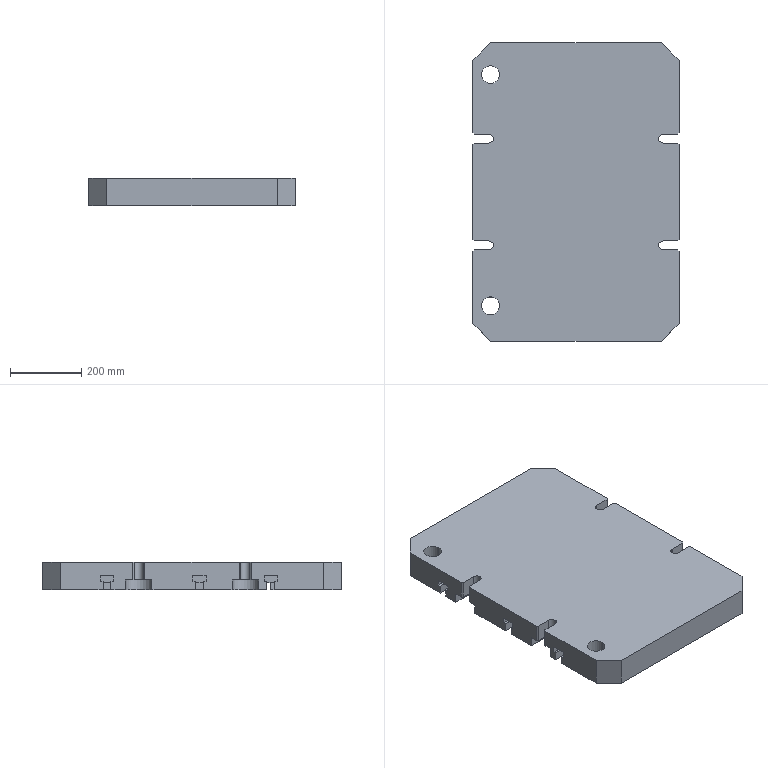Part | 1 solid | 222 faces | box 580 x 840 x 78 mm | volume 31733659 mm3 | plane 106 | cylinder 64 | cone 52 | commonest cylinder face diameters 10 x24 16 x16 6 x12 25 x4 50 x4 75 x4